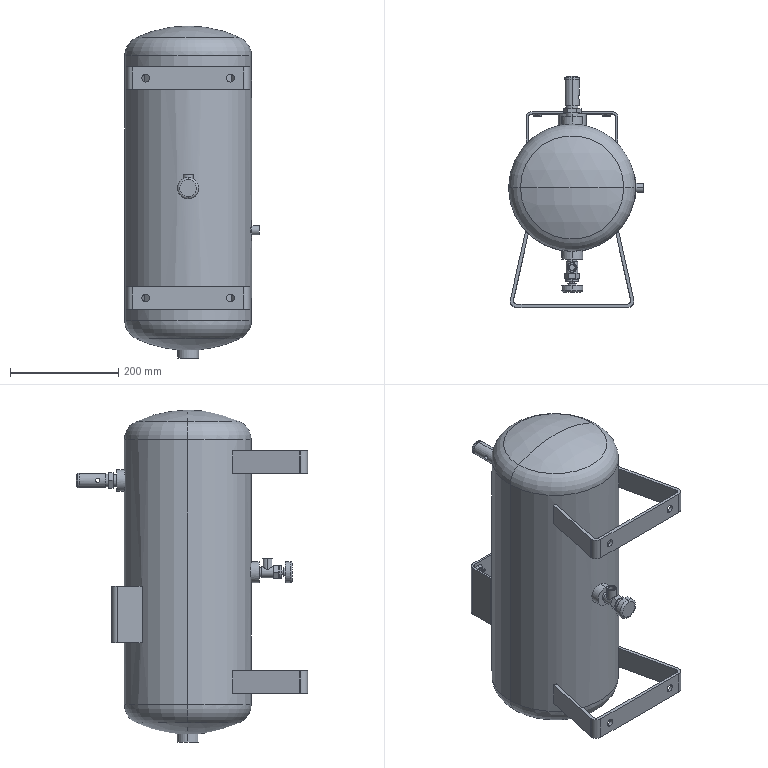Part | SolidWorks | features ICE 2, BaseBody 1, Scale 1 | 1 solid | 233 faces | box 248.43 x 426.53 x 612.3 mm | volume 24721730 mm3 | cylinder 98 | plane 71 | cone 46 | torus 14 | sphere 4 | commonest cylinder face diameters 14.3 x16 39 x10 5.374 x8 10.889 x8 13 x8 24.7 x6